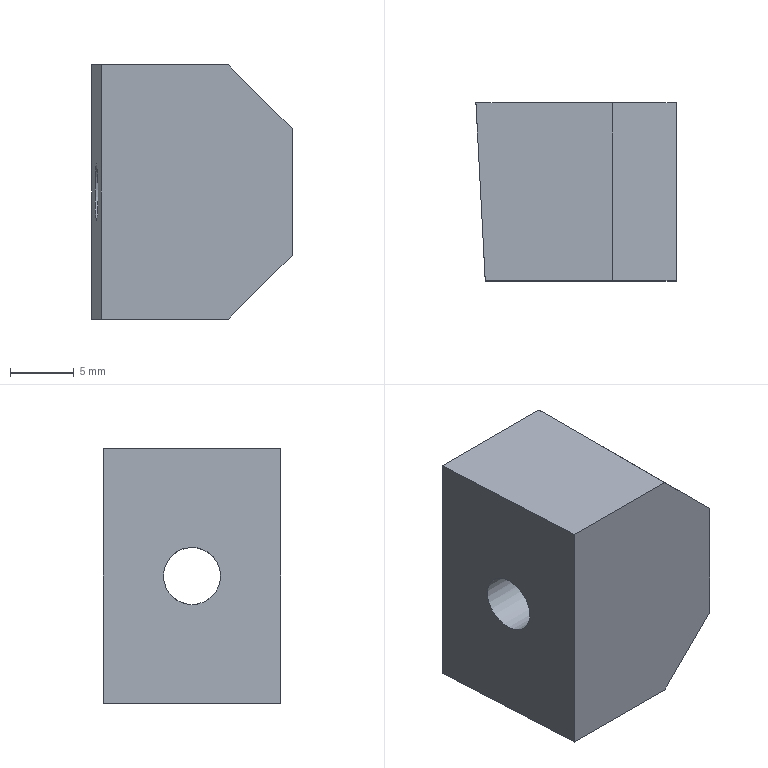Part | STEP file | SLIDE2-INSERT_id70_x_t | 1 solid | 11 faces | box 15.757 x 14 x 20 mm | volume 3560 mm3 | plane 9 | cylinder 2 | commonest cylinder face diameters 4.5 x1 8 x1
STEP:
#1=CARTESIAN_POINT('',(60.5,7.5,132.753));
#2=VERTEX_POINT('',#1);
#3=CARTESIAN_POINT('',(60.5,7.5,135.003));
#4=DIRECTION('',(-1.,0.,0.));
#5=DIRECTION('',(0.,0.,-1.));
#6=AXIS2_PLACEMENT_3D('',#3,#4,#5);
#7=CIRCLE('',#6,2.25);
#8=EDGE_CURVE('',#2,#2,#7,.T.);
#9=ORIENTED_EDGE('',*,*,#8,.T.);
#10=EDGE_LOOP('',(#9));
#11=FACE_BOUND('',#10,.T.);
#12=CARTESIAN_POINT('',(60.5,7.5,131.003));
#13=VERTEX_POINT('',#12);
#14=CARTESIAN_POINT('',(60.5,7.5,135.003));
#15=DIRECTION('',(1.,0.,0.));
#16=DIRECTION('',(0.,0.,-1.));
#17=AXIS2_PLACEMENT_3D('',#14,#15,#16);
#18=CIRCLE('',#17,4.);
#19=EDGE_CURVE('',#13,#13,#18,.T.);
#20=ORIENTED_EDGE('',*,*,#19,.T.);
#21=EDGE_LOOP('',(#20));
#22=FACE_BOUND('',#21,.T.);
#23=CARTESIAN_POINT('',(60.5,-0.5,-265.));
#24=DIRECTION('',(1.,0.,0.));
#25=DIRECTION('',(0.,0.,-1.));
#26=AXIS2_PLACEMENT_3D('',#23,#24,#25);
#27=PLANE('',#26);
#28=ADVANCED_FACE('',(#11,#22),#27,.T.);
#29=ORIENTED_EDGE('',*,*,#19,.F.);
#30=EDGE_LOOP('',(#29));
#31=FACE_BOUND('',#30,.T.);
#32=CARTESIAN_POINT('',(65.,7.5,131.003));
#33=VERTEX_POINT('',#32);
#34=CARTESIAN_POINT('',(65.,7.5,135.003));
#35=DIRECTION('',(-1.,0.,0.));
#36=DIRECTION('',(0.,0.,-1.));
#37=AXIS2_PLACEMENT_3D('',#34,#35,#36);
#38=CIRCLE('',#37,4.);
#39=EDGE_CURVE('',#33,#33,#38,.T.);
#40=ORIENTED_EDGE('',*,*,#39,.F.);
#41=EDGE_LOOP('',(#40));
#42=FACE_BOUND('',#41,.T.);
#43=CARTESIAN_POINT('',(65.,7.5,135.003));
#44=DIRECTION('',(1.,0.,0.));
#45=DIRECTION('',(0.,0.,-1.));
#46=AXIS2_PLACEMENT_3D('',#43,#44,#45);
#47=CYLINDRICAL_SURFACE('',#46,4.);
#48=ADVANCED_FACE('',(#31,#42),#47,.F.);
#49=CARTESIAN_POINT('',(49.728,5.25,135.003));
#50=VERTEX_POINT('',#49);
#51=CARTESIAN_POINT('',(49.61,7.5,135.003));
#52=DIRECTION('',(0.9986,0.05234,0.));
#53=DIRECTION('',(0.05234,-0.9986,0.));
#54=AXIS2_PLACEMENT_3D('',#51,#52,#53);
#55=ELLIPSE('',#54,2.253,2.25);
#56=EDGE_CURVE('',#50,#50,#55,.T.);
#57=ORIENTED_EDGE('',*,*,#56,.F.);
#58=EDGE_LOOP('',(#57));
#59=FACE_BOUND('',#58,.T.);
#60=ORIENTED_EDGE('',*,*,#8,.F.);
#61=EDGE_LOOP('',(#60));
#62=FACE_BOUND('',#61,.T.);
#63=CARTESIAN_POINT('',(65.,7.5,135.003));
#64=DIRECTION('',(1.,0.,0.));
#65=DIRECTION('',(0.,0.,-1.));
#66=AXIS2_PLACEMENT_3D('',#63,#64,#65);
#67=CYLINDRICAL_SURFACE('',#66,2.25);
#68=ADVANCED_FACE('',(#59,#62),#67,.F.);
#69=CARTESIAN_POINT('',(65.,0.5,140.003));
#70=VERTEX_POINT('',#69);
#71=CARTESIAN_POINT('',(60.,0.5,145.003));
#72=VERTEX_POINT('',#71);
#73=CARTESIAN_POINT('',(60.,0.5,145.003));
#74=DIRECTION('',(-0.7071,0.,0.7071));
#75=VECTOR('',#74,1.);
#76=LINE('',#73,#75);
#77=EDGE_CURVE('',#70,#72,#76,.T.);
#78=ORIENTED_EDGE('',*,*,#77,.T.);
#79=CARTESIAN_POINT('',(49.977,0.5,145.003));
#80=VERTEX_POINT('',#79);
#81=CARTESIAN_POINT('',(65.,0.5,145.003));
#82=DIRECTION('',(1.,0.,0.));
#83=VECTOR('',#82,1.);
#84=LINE('',#81,#83);
#85=EDGE_CURVE('',#80,#72,#84,.T.);
#86=ORIENTED_EDGE('',*,*,#85,.F.);
#87=CARTESIAN_POINT('',(49.977,0.5,125.003));
#88=VERTEX_POINT('',#87);
#89=CARTESIAN_POINT('',(49.977,0.5,285.));
#90=DIRECTION('',(0.,0.,1.));
#91=VECTOR('',#90,1.);
#92=LINE('',#89,#91);
#93=EDGE_CURVE('',#88,#80,#92,.T.);
#94=ORIENTED_EDGE('',*,*,#93,.F.);
#95=CARTESIAN_POINT('',(60.,0.5,125.003));
#96=VERTEX_POINT('',#95);
#97=CARTESIAN_POINT('',(-82.114,0.5,125.003));
#98=DIRECTION('',(-1.,0.,0.));
#99=VECTOR('',#98,1.);
#100=LINE('',#97,#99);
#101=EDGE_CURVE('',#96,#88,#100,.T.);
#102=ORIENTED_EDGE('',*,*,#101,.F.);
#103=CARTESIAN_POINT('',(65.,0.5,130.003));
#104=VERTEX_POINT('',#103);
#105=CARTESIAN_POINT('',(65.,0.5,130.003));
#106=DIRECTION('',(0.7071,0.,0.7071));
#107=VECTOR('',#106,1.);
#108=LINE('',#105,#107);
#109=EDGE_CURVE('',#96,#104,#108,.T.);
#110=ORIENTED_EDGE('',*,*,#109,.T.);
#111=CARTESIAN_POINT('',(65.,0.5,125.003));
#112=DIRECTION('',(0.,0.,-1.));
#113=VECTOR('',#112,1.);
#114=LINE('',#111,#113);
#115=EDGE_CURVE('',#70,#104,#114,.T.);
#116=ORIENTED_EDGE('',*,*,#115,.F.);
#117=EDGE_LOOP('',(#78,#86,#94,#102,#110,#116));
#118=FACE_OUTER_BOUND('',#117,.T.);
#119=CARTESIAN_POINT('',(49.977,0.5,285.));
#120=DIRECTION('',(0.,-1.,0.));
#121=DIRECTION('',(0.,0.,-1.));
#122=AXIS2_PLACEMENT_3D('',#119,#120,#121);
#123=PLANE('',#122);
#124=ADVANCED_FACE('',(#118),#123,.T.);
#125=CARTESIAN_POINT('',(65.,14.5,140.003));
#126=VERTEX_POINT('',#125);
#127=CARTESIAN_POINT('',(65.,-0.5,140.003));
#128=DIRECTION('',(0.,-1.,0.));
#129=VECTOR('',#128,1.);
#130=LINE('',#127,#129);
#131=EDGE_CURVE('',#126,#70,#130,.T.);
#132=ORIENTED_EDGE('',*,*,#131,.F.);
#133=CARTESIAN_POINT('',(60.,14.5,145.003));
#134=VERTEX_POINT('',#133);
#135=CARTESIAN_POINT('',(60.,14.5,145.003));
#136=DIRECTION('',(0.7071,0.,-0.7071));
#137=VECTOR('',#136,1.);
#138=LINE('',#135,#137);
#139=EDGE_CURVE('',#134,#126,#138,.T.);
#140=ORIENTED_EDGE('',*,*,#139,.F.);
#141=CARTESIAN_POINT('',(60.,-0.5,145.003));
#142=DIRECTION('',(0.,1.,0.));
#143=VECTOR('',#142,1.);
#144=LINE('',#141,#143);
#145=EDGE_CURVE('',#72,#134,#144,.T.);
#146=ORIENTED_EDGE('',*,*,#145,.F.);
#147=ORIENTED_EDGE('',*,*,#77,.F.);
#148=EDGE_LOOP('',(#132,#140,#146,#147));
#149=FACE_OUTER_BOUND('',#148,.T.);
#150=CARTESIAN_POINT('',(60.,0.5,145.003));
#151=DIRECTION('',(-0.7071,0.,-0.7071));
#152=DIRECTION('',(-0.7071,0.,0.7071));
#153=AXIS2_PLACEMENT_3D('',#150,#151,#152);
#154=PLANE('',#153);
#155=ADVANCED_FACE('',(#149),#154,.F.);
#156=ORIENTED_EDGE('',*,*,#39,.T.);
#157=EDGE_LOOP('',(#156));
#158=FACE_BOUND('',#157,.T.);
#159=CARTESIAN_POINT('',(65.,14.5,130.003));
#160=VERTEX_POINT('',#159);
#161=CARTESIAN_POINT('',(65.,0.5,130.003));
#162=DIRECTION('',(0.,1.,0.));
#163=VECTOR('',#162,1.);
#164=LINE('',#161,#163);
#165=EDGE_CURVE('',#104,#160,#164,.T.);
#166=ORIENTED_EDGE('',*,*,#165,.T.);
#167=CARTESIAN_POINT('',(65.,14.5,285.));
#168=DIRECTION('',(0.,0.,-1.));
#169=VECTOR('',#168,1.);
#170=LINE('',#167,#169);
#171=EDGE_CURVE('',#126,#160,#170,.T.);
#172=ORIENTED_EDGE('',*,*,#171,.F.);
#173=ORIENTED_EDGE('',*,*,#131,.T.);
#174=ORIENTED_EDGE('',*,*,#115,.T.);
#175=EDGE_LOOP('',(#166,#172,#173,#174));
#176=FACE_BOUND('',#175,.T.);
#177=CARTESIAN_POINT('',(65.,-0.5,125.003));
#178=DIRECTION('',(1.,0.,0.));
#179=DIRECTION('',(0.,0.,-1.));
#180=AXIS2_PLACEMENT_3D('',#177,#178,#179);
#181=PLANE('',#180);
#182=ADVANCED_FACE('',(#158,#176),#181,.T.);
#183=CARTESIAN_POINT('',(60.,14.5,125.003));
#184=VERTEX_POINT('',#183);
#185=CARTESIAN_POINT('',(60.,-0.5,125.003));
#186=DIRECTION('',(0.,-1.,0.));
#187=VECTOR('',#186,1.);
#188=LINE('',#185,#187);
#189=EDGE_CURVE('',#184,#96,#188,.T.);
#190=ORIENTED_EDGE('',*,*,#189,.F.);
#191=CARTESIAN_POINT('',(65.,14.5,130.003));
#192=DIRECTION('',(-0.7071,0.,-0.7071));
#193=VECTOR('',#192,1.);
#194=LINE('',#191,#193);
#195=EDGE_CURVE('',#160,#184,#194,.T.);
#196=ORIENTED_EDGE('',*,*,#195,.F.);
#197=ORIENTED_EDGE('',*,*,#165,.F.);
#198=ORIENTED_EDGE('',*,*,#109,.F.);
#199=EDGE_LOOP('',(#190,#196,#197,#198));
#200=FACE_OUTER_BOUND('',#199,.T.);
#201=CARTESIAN_POINT('',(65.,0.5,130.003));
#202=DIRECTION('',(-0.7071,0.,0.7071));
#203=DIRECTION('',(0.7071,0.,0.7071));
#204=AXIS2_PLACEMENT_3D('',#201,#202,#203);
#205=PLANE('',#204);
#206=ADVANCED_FACE('',(#200),#205,.F.);
#207=CARTESIAN_POINT('',(49.243,14.5,125.003));
#208=VERTEX_POINT('',#207);
#209=CARTESIAN_POINT('',(49.243,14.5,125.003));
#210=DIRECTION('',(0.05234,-0.9986,0.));
#211=VECTOR('',#210,1.);
#212=LINE('',#209,#211);
#213=EDGE_CURVE('',#208,#88,#212,.T.);
#214=ORIENTED_EDGE('',*,*,#213,.F.);
#215=CARTESIAN_POINT('',(166.,14.5,125.003));
#216=DIRECTION('',(-1.,0.,0.));
#217=VECTOR('',#216,1.);
#218=LINE('',#215,#217);
#219=EDGE_CURVE('',#184,#208,#218,.T.);
#220=ORIENTED_EDGE('',*,*,#219,.F.);
#221=ORIENTED_EDGE('',*,*,#189,.T.);
#222=ORIENTED_EDGE('',*,*,#101,.T.);
#223=EDGE_LOOP('',(#214,#220,#221,#222));
#224=FACE_OUTER_BOUND('',#223,.T.);
#225=CARTESIAN_POINT('',(-82.114,-0.5,125.003));
#226=DIRECTION('',(0.,0.,-1.));
#227=DIRECTION('',(-1.,0.,0.));
#228=AXIS2_PLACEMENT_3D('',#225,#226,#227);
#229=PLANE('',#228);
#230=ADVANCED_FACE('',(#224),#229,.T.);
#231=ORIENTED_EDGE('',*,*,#56,.T.);
#232=EDGE_LOOP('',(#231));
#233=FACE_BOUND('',#232,.T.);
#234=ORIENTED_EDGE('',*,*,#93,.T.);
#235=CARTESIAN_POINT('',(49.243,14.5,145.003));
#236=VERTEX_POINT('',#235);
#237=CARTESIAN_POINT('',(49.243,14.5,145.003));
#238=DIRECTION('',(0.05234,-0.9986,0.));
#239=VECTOR('',#238,1.);
#240=LINE('',#237,#239);
#241=EDGE_CURVE('',#236,#80,#240,.T.);
#242=ORIENTED_EDGE('',*,*,#241,.F.);
#243=CARTESIAN_POINT('',(49.243,14.5,285.));
#244=DIRECTION('',(0.,0.,1.));
#245=VECTOR('',#244,1.);
#246=LINE('',#243,#245);
#247=EDGE_CURVE('',#208,#236,#246,.T.);
#248=ORIENTED_EDGE('',*,*,#247,.F.);
#249=ORIENTED_EDGE('',*,*,#213,.T.);
#250=EDGE_LOOP('',(#234,#242,#248,#249));
#251=FACE_BOUND('',#250,.T.);
#252=CARTESIAN_POINT('',(49.243,14.5,285.));
#253=DIRECTION('',(-0.9986,-0.05234,0.));
#254=DIRECTION('',(0.05234,-0.9986,0.));
#255=AXIS2_PLACEMENT_3D('',#252,#253,#254);
#256=PLANE('',#255);
#257=ADVANCED_FACE('',(#233,#251),#256,.T.);
#258=ORIENTED_EDGE('',*,*,#145,.T.);
#259=CARTESIAN_POINT('',(166.,14.5,145.003));
#260=DIRECTION('',(1.,0.,0.));
#261=VECTOR('',#260,1.);
#262=LINE('',#259,#261);
#263=EDGE_CURVE('',#236,#134,#262,.T.);
#264=ORIENTED_EDGE('',*,*,#263,.F.);
#265=ORIENTED_EDGE('',*,*,#241,.T.);
#266=ORIENTED_EDGE('',*,*,#85,.T.);
#267=EDGE_LOOP('',(#258,#264,#265,#266));
#268=FACE_OUTER_BOUND('',#267,.T.);
#269=CARTESIAN_POINT('',(65.,-0.5,145.003));
#270=DIRECTION('',(0.,0.,1.));
#271=DIRECTION('',(1.,0.,0.));
#272=AXIS2_PLACEMENT_3D('',#269,#270,#271);
#273=PLANE('',#272);
#274=ADVANCED_FACE('',(#268),#273,.T.);
#275=ORIENTED_EDGE('',*,*,#247,.T.);
#276=ORIENTED_EDGE('',*,*,#263,.T.);
#277=ORIENTED_EDGE('',*,*,#139,.T.);
#278=ORIENTED_EDGE('',*,*,#171,.T.);
#279=ORIENTED_EDGE('',*,*,#195,.T.);
#280=ORIENTED_EDGE('',*,*,#219,.T.);
#281=EDGE_LOOP('',(#275,#276,#277,#278,#279,#280));
#282=FACE_OUTER_BOUND('',#281,.T.);
#283=CARTESIAN_POINT('',(166.,14.5,285.));
#284=DIRECTION('',(0.,1.,0.));
#285=DIRECTION('',(0.,0.,1.));
#286=AXIS2_PLACEMENT_3D('',#283,#284,#285);
#287=PLANE('',#286);
#288=ADVANCED_FACE('',(#282),#287,.T.);
#289=CLOSED_SHELL('',(#28,#48,#68,#124,#155,#182,#206,#230,#257,#274,#288));
#290=MANIFOLD_SOLID_BREP('',#289);
#291=(LENGTH_UNIT()NAMED_UNIT(*)SI_UNIT(.MILLI.,.METRE.));
#292=UNCERTAINTY_MEASURE_WITH_UNIT(LENGTH_MEASURE(0.00002),#291,'','');
#293=(NAMED_UNIT(*)PLANE_ANGLE_UNIT()SI_UNIT($,.RADIAN.));
#294=PLANE_ANGLE_MEASURE_WITH_UNIT(PLANE_ANGLE_MEASURE(0.01745),#293);
#295=DIMENSIONAL_EXPONENTS(0.,0.,0.,0.,0.,0.,0.);
#296=(CONVERSION_BASED_UNIT('DEGREE',#294)NAMED_UNIT(#295)PLANE_ANGLE_UNIT());
#297=(NAMED_UNIT(*)SI_UNIT($,.STERADIAN.)SOLID_ANGLE_UNIT());
#298=(GEOMETRIC_REPRESENTATION_CONTEXT(3)GLOBAL_UNCERTAINTY_ASSIGNED_CONTEXT((#292))GLOBAL_UNIT_ASSIGNED_CONTEXT((#291,#296,#297))REPRESENTATION_CONTEXT('',''));
#299=ADVANCED_BREP_SHAPE_REPRESENTATION('',(#290),#298);